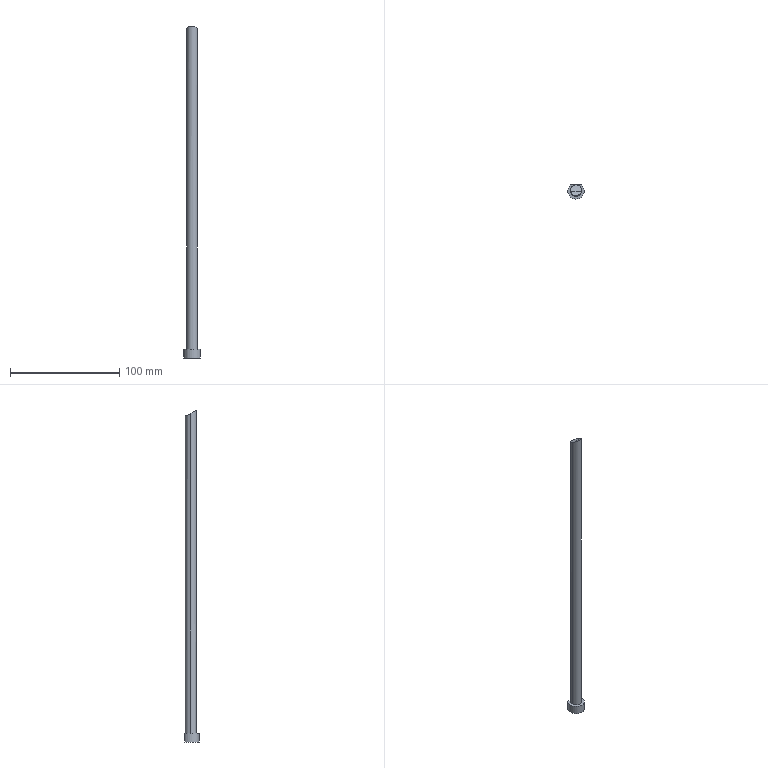Part | Creo | 1 solid | 8 faces | box 15 x 13 x 303.353 mm | volume 24260 mm3 | plane 4 | cylinder 3 | other 1 | commonest cylinder face diameters 10 x2 15 x1
STEP:
#1=CARTESIAN_POINT('',(0.,0.,0.));
#2=DIRECTION('',(0.,0.,1.));
#3=DIRECTION('',(1.,0.,0.));
#4=AXIS2_PLACEMENT_3D('',#1,#2,#3);
#5=CARTESIAN_POINT('',(59.142,71.817,-330.441));
#6=VERTEX_POINT('',#5);
#7=CARTESIAN_POINT('',(48.944,71.817,-330.441));
#8=VERTEX_POINT('',#7);
#9=CARTESIAN_POINT('',(59.142,71.817,-330.441));
#10=DIRECTION('',(-1.,0.,0.));
#11=VECTOR('',#10,10.198);
#12=LINE('',#9,#11);
#13=EDGE_CURVE('',#6,#8,#12,.T.);
#14=ORIENTED_EDGE('',*,*,#13,.F.);
#15=CARTESIAN_POINT('',(54.043,66.317,-330.441));
#16=DIRECTION('',(0.,0.,-1.));
#17=DIRECTION('',(0.6799,0.7333,0.));
#18=AXIS2_PLACEMENT_3D('',#15,#16,#17);
#19=CIRCLE('',#18,7.5);
#20=EDGE_CURVE('',#6,#8,#19,.T.);
#21=ORIENTED_EDGE('',*,*,#20,.T.);
#22=EDGE_LOOP('',(#14,#21));
#23=FACE_OUTER_BOUND('',#22,.F.);
#24=CARTESIAN_POINT('',(49.043,66.317,-330.441));
#25=VERTEX_POINT('',#24);
#26=CARTESIAN_POINT('',(59.043,66.317,-330.441));
#27=VERTEX_POINT('',#26);
#28=CARTESIAN_POINT('',(54.043,66.317,-330.441));
#29=DIRECTION('',(0.,0.,-1.));
#30=DIRECTION('',(-1.,0.,0.));
#31=AXIS2_PLACEMENT_3D('',#28,#29,#30);
#32=CIRCLE('',#31,5.);
#33=EDGE_CURVE('',#25,#27,#32,.T.);
#34=ORIENTED_EDGE('',*,*,#33,.F.);
#35=CARTESIAN_POINT('',(54.043,66.317,-330.441));
#36=DIRECTION('',(0.,0.,-1.));
#37=DIRECTION('',(1.,0.,0.));
#38=AXIS2_PLACEMENT_3D('',#35,#36,#37);
#39=CIRCLE('',#38,5.);
#40=EDGE_CURVE('',#27,#25,#39,.T.);
#41=ORIENTED_EDGE('',*,*,#40,.F.);
#42=EDGE_LOOP('',(#34,#41));
#43=FACE_BOUND('',#42,.F.);
#44=CARTESIAN_POINT('',(54.043,66.317,-330.441));
#45=DIRECTION('',(0.,0.,-1.));
#46=DIRECTION('',(-1.,0.,0.));
#47=AXIS2_PLACEMENT_3D('',#44,#45,#46);
#48=PLANE('',#47);
#49=ADVANCED_FACE('',(#23,#43),#48,.F.);
#50=CARTESIAN_POINT('',(59.043,66.316,-38.277));
#51=VERTEX_POINT('',#50);
#52=CARTESIAN_POINT('',(49.043,66.316,-38.28));
#53=VERTEX_POINT('',#52);
#54=CARTESIAN_POINT('',(59.043,66.316,-38.277));
#55=CARTESIAN_POINT('',(59.043,66.806,-38.558));
#56=CARTESIAN_POINT('',(58.901,67.777,-39.075));
#57=CARTESIAN_POINT('',(58.269,69.123,-39.672));
#58=CARTESIAN_POINT('',(57.286,70.213,-40.089));
#59=CARTESIAN_POINT('',(56.077,70.955,-40.34));
#60=CARTESIAN_POINT('',(54.746,71.332,-40.458));
#61=CARTESIAN_POINT('',(53.34,71.335,-40.459));
#62=CARTESIAN_POINT('',(51.972,70.94,-40.335));
#63=CARTESIAN_POINT('',(50.782,70.193,-40.081));
#64=CARTESIAN_POINT('',(49.83,69.135,-39.677));
#65=CARTESIAN_POINT('',(49.194,67.806,-39.088));
#66=CARTESIAN_POINT('',(49.043,66.819,-38.568));
#67=CARTESIAN_POINT('',(49.043,66.316,-38.28));
#68=B_SPLINE_CURVE_WITH_KNOTS('',3,(#54,#55,#56,#57,#58,#59,#60,#61,#62,#63,#64,#65,#66,#67),.UNSPECIFIED.,.F.,.F.,(4,1,1,1,1,1,1,1,1,1,1,4),(0.,0.09091,0.1818,0.2727,0.3636,0.4545,0.5455,0.6364,0.7273,0.8182,0.9091,1.),.UNSPECIFIED.);
#69=EDGE_CURVE('',#51,#53,#68,.T.);
#70=ORIENTED_EDGE('',*,*,#69,.T.);
#71=CARTESIAN_POINT('',(49.043,66.317,-330.441));
#72=DIRECTION('',(-0.000001619,-0.000003335,1.));
#73=VECTOR('',#72,292.162);
#74=LINE('',#71,#73);
#75=EDGE_CURVE('',#25,#53,#74,.T.);
#76=ORIENTED_EDGE('',*,*,#75,.F.);
#77=ORIENTED_EDGE('',*,*,#33,.T.);
#78=CARTESIAN_POINT('',(59.043,66.317,-330.441));
#79=DIRECTION('',(-0.000000893,-0.000003722,1.));
#80=VECTOR('',#79,292.164);
#81=LINE('',#78,#80);
#82=EDGE_CURVE('',#27,#51,#81,.T.);
#83=ORIENTED_EDGE('',*,*,#82,.T.);
#84=EDGE_LOOP('',(#70,#76,#77,#83));
#85=FACE_OUTER_BOUND('',#84,.F.);
#86=CARTESIAN_POINT('',(54.043,66.317,-653.441));
#87=DIRECTION('',(0.,0.,1.));
#88=DIRECTION('',(1.,0.,0.));
#89=AXIS2_PLACEMENT_3D('',#86,#87,#88);
#90=CYLINDRICAL_SURFACE('',#89,5.);
#91=ADVANCED_FACE('',(#85),#90,.T.);
#92=CARTESIAN_POINT('',(49.173,65.184,-37.592));
#93=VERTEX_POINT('',#92);
#94=CARTESIAN_POINT('',(58.913,65.184,-37.592));
#95=VERTEX_POINT('',#94);
#96=CARTESIAN_POINT('',(49.173,65.184,-37.592));
#97=DIRECTION('',(1.,0.,0.));
#98=VECTOR('',#97,9.74);
#99=LINE('',#96,#98);
#100=EDGE_CURVE('',#93,#95,#99,.T.);
#101=ORIENTED_EDGE('',*,*,#100,.F.);
#102=CARTESIAN_POINT('',(49.043,66.316,-38.28));
#103=CARTESIAN_POINT('',(49.043,66.116,-38.165));
#104=CARTESIAN_POINT('',(49.067,65.728,-37.939));
#105=CARTESIAN_POINT('',(49.132,65.361,-37.707));
#106=CARTESIAN_POINT('',(49.173,65.184,-37.592));
#107=B_SPLINE_CURVE_WITH_KNOTS('',3,(#102,#103,#104,#105,#106),.UNSPECIFIED.,.F.,.F.,(4,1,4),(0.,0.5,1.),.UNSPECIFIED.);
#108=EDGE_CURVE('',#53,#93,#107,.T.);
#109=ORIENTED_EDGE('',*,*,#108,.F.);
#110=ORIENTED_EDGE('',*,*,#69,.F.);
#111=CARTESIAN_POINT('',(58.913,65.184,-37.592));
#112=CARTESIAN_POINT('',(58.955,65.364,-37.708));
#113=CARTESIAN_POINT('',(59.02,65.731,-37.942));
#114=CARTESIAN_POINT('',(59.043,66.12,-38.165));
#115=CARTESIAN_POINT('',(59.043,66.316,-38.277));
#116=B_SPLINE_CURVE_WITH_KNOTS('',3,(#111,#112,#113,#114,#115),.UNSPECIFIED.,.F.,.F.,(4,1,4),(0.,0.5,1.),.UNSPECIFIED.);
#117=EDGE_CURVE('',#95,#51,#116,.T.);
#118=ORIENTED_EDGE('',*,*,#117,.F.);
#119=EDGE_LOOP('',(#101,#109,#110,#118));
#120=FACE_OUTER_BOUND('',#119,.F.);
#121=CARTESIAN_POINT('',(19.953,65.024,-37.488));
#122=CARTESIAN_POINT('',(19.953,67.005,-38.792));
#123=CARTESIAN_POINT('',(19.953,69.162,-39.799));
#124=CARTESIAN_POINT('',(19.953,71.495,-40.508));
#125=B_SPLINE_CURVE_WITH_KNOTS('',3,(#121,#122,#123,#124),.UNSPECIFIED.,.F.,.F.,(4,4),(0.,1.),.UNSPECIFIED.);
#126=DIRECTION('',(1.,0.,0.));
#127=VECTOR('',#126,1.);
#128=SURFACE_OF_LINEAR_EXTRUSION('',#125,#127);
#129=ADVANCED_FACE('',(#120),#128,.F.);
#130=ORIENTED_EDGE('',*,*,#100,.T.);
#131=CARTESIAN_POINT('',(56.725,62.098,-35.594));
#132=VERTEX_POINT('',#131);
#133=CARTESIAN_POINT('',(56.725,62.098,-35.594));
#134=CARTESIAN_POINT('',(57.334,62.484,-35.844));
#135=CARTESIAN_POINT('',(58.252,63.414,-36.446));
#136=CARTESIAN_POINT('',(58.767,64.555,-37.185));
#137=CARTESIAN_POINT('',(58.913,65.184,-37.592));
#138=B_SPLINE_CURVE_WITH_KNOTS('',3,(#133,#134,#135,#136,#137),.UNSPECIFIED.,.F.,.F.,(4,1,4),(0.,0.5,1.),.UNSPECIFIED.);
#139=EDGE_CURVE('',#132,#95,#138,.T.);
#140=ORIENTED_EDGE('',*,*,#139,.F.);
#141=CARTESIAN_POINT('',(49.173,65.184,-37.592));
#142=CARTESIAN_POINT('',(49.3,64.641,-37.241));
#143=CARTESIAN_POINT('',(49.665,63.803,-36.698));
#144=CARTESIAN_POINT('',(50.594,62.566,-35.898));
#145=CARTESIAN_POINT('',(52.022,61.603,-35.274));
#146=CARTESIAN_POINT('',(53.717,61.227,-35.031));
#147=CARTESIAN_POINT('',(55.3,61.425,-35.159));
#148=CARTESIAN_POINT('',(56.2,61.764,-35.378));
#149=B_SPLINE_CURVE_WITH_KNOTS('',3,(#141,#142,#143,#144,#145,#146,#147,#148,#131),.UNSPECIFIED.,.F.,.F.,(4,1,1,1,1,1,4),(0.,0.125,0.25,0.5,0.75,0.875,1.),.UNSPECIFIED.);
#150=EDGE_CURVE('',#93,#132,#149,.T.);
#151=ORIENTED_EDGE('',*,*,#150,.F.);
#152=EDGE_LOOP('',(#130,#140,#151));
#153=FACE_OUTER_BOUND('',#152,.F.);
#154=CARTESIAN_POINT('',(20.453,63.212,-36.316));
#155=DIRECTION('',(0.,0.5434,0.8395));
#156=DIRECTION('',(0.,0.8395,-0.5434));
#157=AXIS2_PLACEMENT_3D('',#154,#155,#156);
#158=PLANE('',#157);
#159=ADVANCED_FACE('',(#153),#158,.T.);
#160=ORIENTED_EDGE('',*,*,#108,.T.);
#161=ORIENTED_EDGE('',*,*,#150,.T.);
#162=ORIENTED_EDGE('',*,*,#139,.T.);
#163=ORIENTED_EDGE('',*,*,#117,.T.);
#164=ORIENTED_EDGE('',*,*,#82,.F.);
#165=ORIENTED_EDGE('',*,*,#40,.T.);
#166=ORIENTED_EDGE('',*,*,#75,.T.);
#167=EDGE_LOOP('',(#160,#161,#162,#163,#164,#165,#166));
#168=FACE_OUTER_BOUND('',#167,.F.);
#169=CARTESIAN_POINT('',(54.043,66.317,-653.441));
#170=DIRECTION('',(0.,0.,1.));
#171=DIRECTION('',(1.,0.,0.));
#172=AXIS2_PLACEMENT_3D('',#169,#170,#171);
#173=CYLINDRICAL_SURFACE('',#172,5.);
#174=ADVANCED_FACE('',(#168),#173,.T.);
#175=CARTESIAN_POINT('',(48.944,71.817,-338.441));
#176=VERTEX_POINT('',#175);
#177=CARTESIAN_POINT('',(48.944,71.817,-330.441));
#178=DIRECTION('',(0.,0.,-1.));
#179=VECTOR('',#178,8.);
#180=LINE('',#177,#179);
#181=EDGE_CURVE('',#8,#176,#180,.T.);
#182=ORIENTED_EDGE('',*,*,#181,.T.);
#183=CARTESIAN_POINT('',(59.142,71.817,-338.441));
#184=VERTEX_POINT('',#183);
#185=CARTESIAN_POINT('',(59.142,71.817,-338.441));
#186=DIRECTION('',(-1.,0.,0.));
#187=VECTOR('',#186,10.198);
#188=LINE('',#185,#187);
#189=EDGE_CURVE('',#184,#176,#188,.T.);
#190=ORIENTED_EDGE('',*,*,#189,.F.);
#191=CARTESIAN_POINT('',(59.142,71.817,-338.441));
#192=DIRECTION('',(0.,0.,1.));
#193=VECTOR('',#192,8.);
#194=LINE('',#191,#193);
#195=EDGE_CURVE('',#184,#6,#194,.T.);
#196=ORIENTED_EDGE('',*,*,#195,.T.);
#197=ORIENTED_EDGE('',*,*,#13,.T.);
#198=EDGE_LOOP('',(#182,#190,#196,#197));
#199=FACE_OUTER_BOUND('',#198,.F.);
#200=CARTESIAN_POINT('',(54.043,71.817,-338.441));
#201=DIRECTION('',(0.,1.,0.));
#202=DIRECTION('',(0.,0.,1.));
#203=AXIS2_PLACEMENT_3D('',#200,#201,#202);
#204=PLANE('',#203);
#205=ADVANCED_FACE('',(#199),#204,.T.);
#206=CARTESIAN_POINT('',(54.043,66.317,-338.441));
#207=DIRECTION('',(0.,0.,1.));
#208=DIRECTION('',(-0.6799,0.7333,0.));
#209=AXIS2_PLACEMENT_3D('',#206,#207,#208);
#210=CIRCLE('',#209,7.5);
#211=EDGE_CURVE('',#176,#184,#210,.T.);
#212=ORIENTED_EDGE('',*,*,#211,.F.);
#213=ORIENTED_EDGE('',*,*,#181,.F.);
#214=ORIENTED_EDGE('',*,*,#20,.F.);
#215=ORIENTED_EDGE('',*,*,#195,.F.);
#216=EDGE_LOOP('',(#212,#213,#214,#215));
#217=FACE_OUTER_BOUND('',#216,.F.);
#218=CARTESIAN_POINT('',(54.043,66.317,-330.441));
#219=DIRECTION('',(0.,0.,-1.));
#220=DIRECTION('',(-1.,0.,0.));
#221=AXIS2_PLACEMENT_3D('',#218,#219,#220);
#222=CYLINDRICAL_SURFACE('',#221,7.5);
#223=ADVANCED_FACE('',(#217),#222,.T.);
#224=ORIENTED_EDGE('',*,*,#211,.T.);
#225=ORIENTED_EDGE('',*,*,#189,.T.);
#226=EDGE_LOOP('',(#224,#225));
#227=FACE_OUTER_BOUND('',#226,.F.);
#228=CARTESIAN_POINT('',(54.043,66.317,-338.441));
#229=DIRECTION('',(0.,0.,-1.));
#230=DIRECTION('',(-1.,0.,0.));
#231=AXIS2_PLACEMENT_3D('',#228,#229,#230);
#232=PLANE('',#231);
#233=ADVANCED_FACE('',(#227),#232,.T.);
#234=CLOSED_SHELL('',(#49,#91,#129,#159,#174,#205,#223,#233));
#235=MANIFOLD_SOLID_BREP('',#234);
#236=(LENGTH_UNIT()NAMED_UNIT(*)SI_UNIT(.MILLI.,.METRE.));
#237=UNCERTAINTY_MEASURE_WITH_UNIT(LENGTH_MEASURE(0.0304),#236,'','');
#238=(NAMED_UNIT(*)PLANE_ANGLE_UNIT()SI_UNIT($,.RADIAN.));
#239=PLANE_ANGLE_MEASURE_WITH_UNIT(PLANE_ANGLE_MEASURE(0.01745),#238);
#240=(CONVERSION_BASED_UNIT('DEGREE',#239)NAMED_UNIT(*)PLANE_ANGLE_UNIT());
#241=(NAMED_UNIT(*)SI_UNIT($,.STERADIAN.)SOLID_ANGLE_UNIT());
#242=(GEOMETRIC_REPRESENTATION_CONTEXT(3)GLOBAL_UNCERTAINTY_ASSIGNED_CONTEXT((#237))GLOBAL_UNIT_ASSIGNED_CONTEXT((#236,#240,#241))REPRESENTATION_CONTEXT('',''));
#243=ADVANCED_BREP_SHAPE_REPRESENTATION('',(#4,#235),#242);